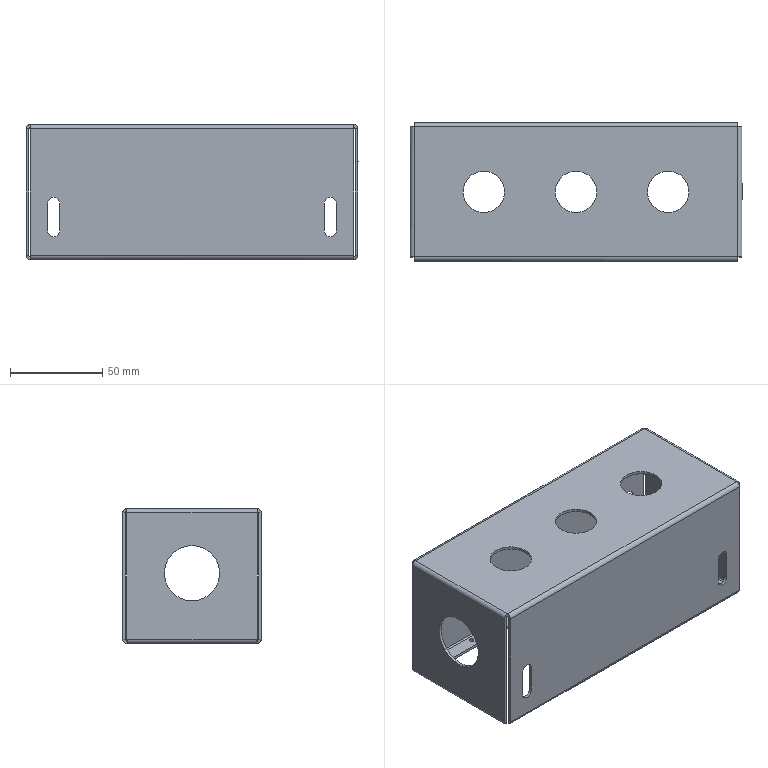Part | NX | 1 solid | 97 faces | box 180 x 75 x 73 mm | volume 72373 mm3 | plane 46 | cylinder 35 | spline 16 | commonest cylinder face diameters 1.473 x8 4.473 x8 2.5 x6 6.5 x4 12 x4 22.5 x3